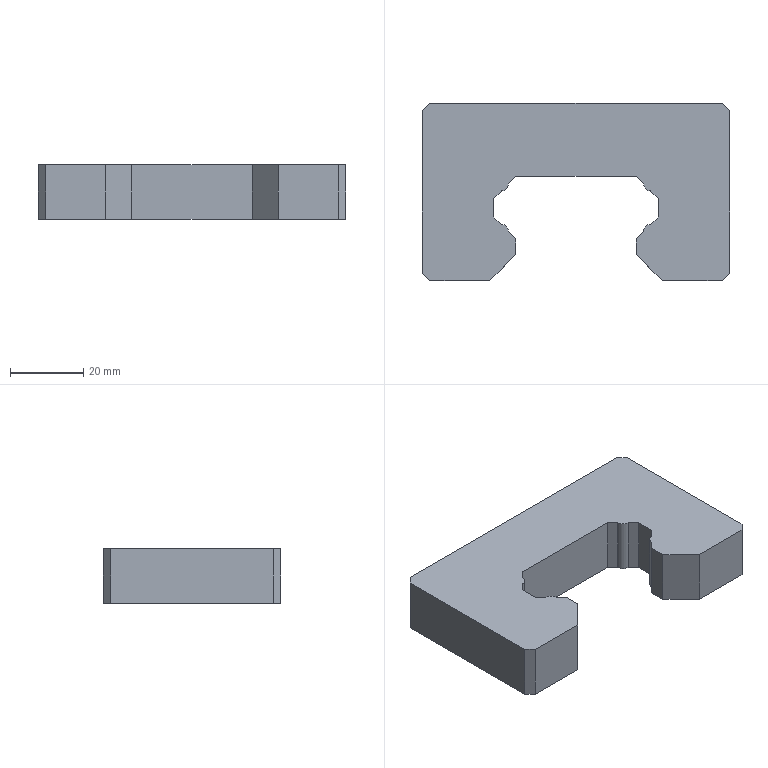Part | SolidWorks | features SplitBody 1 | 1 solid | 32 faces | box 84.105 x 48.48 x 15 mm | volume 44236 mm3 | plane 26 | cylinder 6 | commonest cylinder face diameters 3.924 x6
STEP:
#1=CARTESIAN_POINT('',(-18.51,13.429,79.55));
#2=VERTEX_POINT('',#1);
#3=CARTESIAN_POINT('',(-18.51,13.395,79.55));
#4=VERTEX_POINT('',#3);
#5=CARTESIAN_POINT('',(-20.471,13.429,79.55));
#6=DIRECTION('',(0.,0.,-1.));
#7=DIRECTION('',(-1.,0.,0.));
#8=AXIS2_PLACEMENT_3D('',#5,#6,#7);
#9=CIRCLE('',#8,1.962);
#10=EDGE_CURVE('',#2,#4,#9,.T.);
#11=ORIENTED_EDGE('',*,*,#10,.F.);
#12=CARTESIAN_POINT('',(-18.51,13.429,94.55));
#13=VERTEX_POINT('',#12);
#14=CARTESIAN_POINT('',(-18.51,13.429,79.55));
#15=DIRECTION('',(0.,0.,1.));
#16=VECTOR('',#15,1000.);
#17=LINE('',#14,#16);
#18=EDGE_CURVE('',#2,#13,#17,.T.);
#19=ORIENTED_EDGE('',*,*,#18,.T.);
#20=CARTESIAN_POINT('',(-18.51,13.395,94.55));
#21=VERTEX_POINT('',#20);
#22=CARTESIAN_POINT('',(-20.471,13.429,94.55));
#23=DIRECTION('',(0.,0.,-1.));
#24=DIRECTION('',(-1.,0.,0.));
#25=AXIS2_PLACEMENT_3D('',#22,#23,#24);
#26=CIRCLE('',#25,1.962);
#27=EDGE_CURVE('',#13,#21,#26,.T.);
#28=ORIENTED_EDGE('',*,*,#27,.T.);
#29=CARTESIAN_POINT('',(-18.51,13.395,79.55));
#30=DIRECTION('',(0.,0.,1.));
#31=VECTOR('',#30,1000.);
#32=LINE('',#29,#31);
#33=EDGE_CURVE('',#4,#21,#32,.T.);
#34=ORIENTED_EDGE('',*,*,#33,.F.);
#35=EDGE_LOOP('',(#11,#19,#28,#34));
#36=FACE_OUTER_BOUND('',#35,.T.);
#37=CARTESIAN_POINT('',(-20.471,13.429,79.55));
#38=DIRECTION('',(0.,0.,1.));
#39=DIRECTION('',(1.,0.,0.));
#40=AXIS2_PLACEMENT_3D('',#37,#38,#39);
#41=CYLINDRICAL_SURFACE('',#40,1.962);
#42=ADVANCED_FACE('',(#36),#41,.T.);
#43=CARTESIAN_POINT('',(-18.51,26.471,79.55));
#44=VERTEX_POINT('',#43);
#45=CARTESIAN_POINT('',(-20.505,24.51,79.55));
#46=VERTEX_POINT('',#45);
#47=CARTESIAN_POINT('',(-20.471,26.471,79.55));
#48=DIRECTION('',(0.,0.,-1.));
#49=DIRECTION('',(-1.,0.,0.));
#50=AXIS2_PLACEMENT_3D('',#47,#48,#49);
#51=CIRCLE('',#50,1.962);
#52=EDGE_CURVE('',#44,#46,#51,.T.);
#53=ORIENTED_EDGE('',*,*,#52,.F.);
#54=CARTESIAN_POINT('',(-18.51,26.471,94.55));
#55=VERTEX_POINT('',#54);
#56=CARTESIAN_POINT('',(-18.51,26.471,79.55));
#57=DIRECTION('',(0.,0.,1.));
#58=VECTOR('',#57,1000.);
#59=LINE('',#56,#58);
#60=EDGE_CURVE('',#44,#55,#59,.T.);
#61=ORIENTED_EDGE('',*,*,#60,.T.);
#62=CARTESIAN_POINT('',(-20.505,24.51,94.55));
#63=VERTEX_POINT('',#62);
#64=CARTESIAN_POINT('',(-20.471,26.471,94.55));
#65=DIRECTION('',(0.,0.,-1.));
#66=DIRECTION('',(-1.,0.,0.));
#67=AXIS2_PLACEMENT_3D('',#64,#65,#66);
#68=CIRCLE('',#67,1.962);
#69=EDGE_CURVE('',#55,#63,#68,.T.);
#70=ORIENTED_EDGE('',*,*,#69,.T.);
#71=CARTESIAN_POINT('',(-20.505,24.51,79.55));
#72=DIRECTION('',(0.,0.,1.));
#73=VECTOR('',#72,1000.);
#74=LINE('',#71,#73);
#75=EDGE_CURVE('',#46,#63,#74,.T.);
#76=ORIENTED_EDGE('',*,*,#75,.F.);
#77=EDGE_LOOP('',(#53,#61,#70,#76));
#78=FACE_OUTER_BOUND('',#77,.T.);
#79=CARTESIAN_POINT('',(-20.471,26.471,79.55));
#80=DIRECTION('',(0.,0.,1.));
#81=DIRECTION('',(1.,0.,0.));
#82=AXIS2_PLACEMENT_3D('',#79,#80,#81);
#83=CYLINDRICAL_SURFACE('',#82,1.962);
#84=ADVANCED_FACE('',(#78),#83,.T.);
#85=CARTESIAN_POINT('',(-16.515,11.4,94.55));
#86=VERTEX_POINT('',#85);
#87=CARTESIAN_POINT('',(-16.515,7.11,94.55));
#88=VERTEX_POINT('',#87);
#89=CARTESIAN_POINT('',(-16.515,11.4,94.55));
#90=DIRECTION('',(0.,-1.,0.));
#91=VECTOR('',#90,1000.);
#92=LINE('',#89,#91);
#93=EDGE_CURVE('',#86,#88,#92,.T.);
#94=ORIENTED_EDGE('',*,*,#93,.T.);
#95=CARTESIAN_POINT('',(-16.515,7.11,79.55));
#96=VERTEX_POINT('',#95);
#97=CARTESIAN_POINT('',(-16.515,7.11,79.55));
#98=DIRECTION('',(0.,0.,1.));
#99=VECTOR('',#98,1000.);
#100=LINE('',#97,#99);
#101=EDGE_CURVE('',#96,#88,#100,.T.);
#102=ORIENTED_EDGE('',*,*,#101,.F.);
#103=CARTESIAN_POINT('',(-16.515,11.4,79.55));
#104=VERTEX_POINT('',#103);
#105=CARTESIAN_POINT('',(-16.515,11.4,79.55));
#106=DIRECTION('',(0.,-1.,0.));
#107=VECTOR('',#106,1000.);
#108=LINE('',#105,#107);
#109=EDGE_CURVE('',#104,#96,#108,.T.);
#110=ORIENTED_EDGE('',*,*,#109,.F.);
#111=CARTESIAN_POINT('',(-16.515,11.4,79.55));
#112=DIRECTION('',(0.,0.,1.));
#113=VECTOR('',#112,1000.);
#114=LINE('',#111,#113);
#115=EDGE_CURVE('',#104,#86,#114,.T.);
#116=ORIENTED_EDGE('',*,*,#115,.T.);
#117=EDGE_LOOP('',(#94,#102,#110,#116));
#118=FACE_OUTER_BOUND('',#117,.T.);
#119=CARTESIAN_POINT('',(-16.515,11.4,79.55));
#120=DIRECTION('',(-1.,0.,0.));
#121=DIRECTION('',(0.,-1.,0.));
#122=AXIS2_PLACEMENT_3D('',#119,#120,#121);
#123=PLANE('',#122);
#124=ADVANCED_FACE('',(#118),#123,.F.);
#125=CARTESIAN_POINT('',(-23.625,0.,94.55));
#126=VERTEX_POINT('',#125);
#127=CARTESIAN_POINT('',(-16.515,7.11,94.55));
#128=DIRECTION('',(-0.7071,-0.7071,0.));
#129=VECTOR('',#128,1000.);
#130=LINE('',#127,#129);
#131=EDGE_CURVE('',#88,#126,#130,.T.);
#132=ORIENTED_EDGE('',*,*,#131,.T.);
#133=CARTESIAN_POINT('',(-23.625,0.,79.55));
#134=VERTEX_POINT('',#133);
#135=CARTESIAN_POINT('',(-23.625,0.,79.55));
#136=DIRECTION('',(0.,0.,1.));
#137=VECTOR('',#136,1000.);
#138=LINE('',#135,#137);
#139=EDGE_CURVE('',#134,#126,#138,.T.);
#140=ORIENTED_EDGE('',*,*,#139,.F.);
#141=CARTESIAN_POINT('',(-16.515,7.11,79.55));
#142=DIRECTION('',(-0.7071,-0.7071,0.));
#143=VECTOR('',#142,1000.);
#144=LINE('',#141,#143);
#145=EDGE_CURVE('',#96,#134,#144,.T.);
#146=ORIENTED_EDGE('',*,*,#145,.F.);
#147=ORIENTED_EDGE('',*,*,#101,.T.);
#148=EDGE_LOOP('',(#132,#140,#146,#147));
#149=FACE_OUTER_BOUND('',#148,.T.);
#150=CARTESIAN_POINT('',(-16.515,7.11,79.55));
#151=DIRECTION('',(-0.7071,0.7071,0.));
#152=DIRECTION('',(-0.7071,-0.7071,0.));
#153=AXIS2_PLACEMENT_3D('',#150,#151,#152);
#154=PLANE('',#153);
#155=ADVANCED_FACE('',(#149),#154,.F.);
#156=CARTESIAN_POINT('',(-40.05,0.,94.55));
#157=VERTEX_POINT('',#156);
#158=CARTESIAN_POINT('',(-23.625,0.,94.55));
#159=DIRECTION('',(-1.,0.,0.));
#160=VECTOR('',#159,1000.);
#161=LINE('',#158,#160);
#162=EDGE_CURVE('',#126,#157,#161,.T.);
#163=ORIENTED_EDGE('',*,*,#162,.T.);
#164=CARTESIAN_POINT('',(-40.05,0.,79.55));
#165=VERTEX_POINT('',#164);
#166=CARTESIAN_POINT('',(-40.05,0.,79.55));
#167=DIRECTION('',(0.,0.,1.));
#168=VECTOR('',#167,1000.);
#169=LINE('',#166,#168);
#170=EDGE_CURVE('',#165,#157,#169,.T.);
#171=ORIENTED_EDGE('',*,*,#170,.F.);
#172=CARTESIAN_POINT('',(-23.625,0.,79.55));
#173=DIRECTION('',(-1.,0.,0.));
#174=VECTOR('',#173,1000.);
#175=LINE('',#172,#174);
#176=EDGE_CURVE('',#134,#165,#175,.T.);
#177=ORIENTED_EDGE('',*,*,#176,.F.);
#178=ORIENTED_EDGE('',*,*,#139,.T.);
#179=EDGE_LOOP('',(#163,#171,#177,#178));
#180=FACE_OUTER_BOUND('',#179,.T.);
#181=CARTESIAN_POINT('',(-23.625,0.,79.55));
#182=DIRECTION('',(0.,1.,0.));
#183=DIRECTION('',(-1.,0.,0.));
#184=AXIS2_PLACEMENT_3D('',#181,#182,#183);
#185=PLANE('',#184);
#186=ADVANCED_FACE('',(#180),#185,.F.);
#187=CARTESIAN_POINT('',(-42.053,2.002,94.55));
#188=VERTEX_POINT('',#187);
#189=CARTESIAN_POINT('',(-40.05,0.,94.55));
#190=DIRECTION('',(-0.7071,0.7071,0.));
#191=VECTOR('',#190,1000.);
#192=LINE('',#189,#191);
#193=EDGE_CURVE('',#157,#188,#192,.T.);
#194=ORIENTED_EDGE('',*,*,#193,.T.);
#195=CARTESIAN_POINT('',(-42.053,2.002,79.55));
#196=VERTEX_POINT('',#195);
#197=CARTESIAN_POINT('',(-42.053,2.002,79.55));
#198=DIRECTION('',(0.,0.,1.));
#199=VECTOR('',#198,1000.);
#200=LINE('',#197,#199);
#201=EDGE_CURVE('',#196,#188,#200,.T.);
#202=ORIENTED_EDGE('',*,*,#201,.F.);
#203=CARTESIAN_POINT('',(-40.05,0.,79.55));
#204=DIRECTION('',(-0.7071,0.7071,0.));
#205=VECTOR('',#204,1000.);
#206=LINE('',#203,#205);
#207=EDGE_CURVE('',#165,#196,#206,.T.);
#208=ORIENTED_EDGE('',*,*,#207,.F.);
#209=ORIENTED_EDGE('',*,*,#170,.T.);
#210=EDGE_LOOP('',(#194,#202,#208,#209));
#211=FACE_OUTER_BOUND('',#210,.T.);
#212=CARTESIAN_POINT('',(-40.05,0.,79.55));
#213=DIRECTION('',(0.7071,0.7071,0.));
#214=DIRECTION('',(-0.7071,0.7071,0.));
#215=AXIS2_PLACEMENT_3D('',#212,#213,#214);
#216=PLANE('',#215);
#217=ADVANCED_FACE('',(#211),#216,.F.);
#218=CARTESIAN_POINT('',(-42.053,46.477,94.55));
#219=VERTEX_POINT('',#218);
#220=CARTESIAN_POINT('',(-42.053,2.002,94.55));
#221=DIRECTION('',(0.,1.,0.));
#222=VECTOR('',#221,1000.);
#223=LINE('',#220,#222);
#224=EDGE_CURVE('',#188,#219,#223,.T.);
#225=ORIENTED_EDGE('',*,*,#224,.T.);
#226=CARTESIAN_POINT('',(-42.053,46.477,79.55));
#227=VERTEX_POINT('',#226);
#228=CARTESIAN_POINT('',(-42.053,46.477,79.55));
#229=DIRECTION('',(0.,0.,1.));
#230=VECTOR('',#229,1000.);
#231=LINE('',#228,#230);
#232=EDGE_CURVE('',#227,#219,#231,.T.);
#233=ORIENTED_EDGE('',*,*,#232,.F.);
#234=CARTESIAN_POINT('',(-42.053,2.002,79.55));
#235=DIRECTION('',(0.,1.,0.));
#236=VECTOR('',#235,1000.);
#237=LINE('',#234,#236);
#238=EDGE_CURVE('',#196,#227,#237,.T.);
#239=ORIENTED_EDGE('',*,*,#238,.F.);
#240=ORIENTED_EDGE('',*,*,#201,.T.);
#241=EDGE_LOOP('',(#225,#233,#239,#240));
#242=FACE_OUTER_BOUND('',#241,.T.);
#243=CARTESIAN_POINT('',(-42.053,2.002,79.55));
#244=DIRECTION('',(1.,0.,0.));
#245=DIRECTION('',(0.,0.,-1.));
#246=AXIS2_PLACEMENT_3D('',#243,#244,#245);
#247=PLANE('',#246);
#248=ADVANCED_FACE('',(#242),#247,.F.);
#249=CARTESIAN_POINT('',(-40.05,48.48,94.55));
#250=VERTEX_POINT('',#249);
#251=CARTESIAN_POINT('',(-42.053,46.477,94.55));
#252=DIRECTION('',(0.7071,0.7071,0.));
#253=VECTOR('',#252,1000.);
#254=LINE('',#251,#253);
#255=EDGE_CURVE('',#219,#250,#254,.T.);
#256=ORIENTED_EDGE('',*,*,#255,.T.);
#257=CARTESIAN_POINT('',(-40.05,48.48,79.55));
#258=VERTEX_POINT('',#257);
#259=CARTESIAN_POINT('',(-40.05,48.48,79.55));
#260=DIRECTION('',(0.,0.,1.));
#261=VECTOR('',#260,1000.);
#262=LINE('',#259,#261);
#263=EDGE_CURVE('',#258,#250,#262,.T.);
#264=ORIENTED_EDGE('',*,*,#263,.F.);
#265=CARTESIAN_POINT('',(-42.053,46.477,79.55));
#266=DIRECTION('',(0.7071,0.7071,0.));
#267=VECTOR('',#266,1000.);
#268=LINE('',#265,#267);
#269=EDGE_CURVE('',#227,#258,#268,.T.);
#270=ORIENTED_EDGE('',*,*,#269,.F.);
#271=ORIENTED_EDGE('',*,*,#232,.T.);
#272=EDGE_LOOP('',(#256,#264,#270,#271));
#273=FACE_OUTER_BOUND('',#272,.T.);
#274=CARTESIAN_POINT('',(-42.053,46.477,79.55));
#275=DIRECTION('',(0.7071,-0.7071,0.));
#276=DIRECTION('',(0.7071,0.7071,0.));
#277=AXIS2_PLACEMENT_3D('',#274,#275,#276);
#278=PLANE('',#277);
#279=ADVANCED_FACE('',(#273),#278,.F.);
#280=CARTESIAN_POINT('',(40.05,48.48,94.55));
#281=VERTEX_POINT('',#280);
#282=CARTESIAN_POINT('',(-40.05,48.48,94.55));
#283=DIRECTION('',(1.,0.,0.));
#284=VECTOR('',#283,1000.);
#285=LINE('',#282,#284);
#286=EDGE_CURVE('',#250,#281,#285,.T.);
#287=ORIENTED_EDGE('',*,*,#286,.T.);
#288=CARTESIAN_POINT('',(40.05,48.48,79.55));
#289=VERTEX_POINT('',#288);
#290=CARTESIAN_POINT('',(40.05,48.48,79.55));
#291=DIRECTION('',(0.,0.,1.));
#292=VECTOR('',#291,1000.);
#293=LINE('',#290,#292);
#294=EDGE_CURVE('',#289,#281,#293,.T.);
#295=ORIENTED_EDGE('',*,*,#294,.F.);
#296=CARTESIAN_POINT('',(-40.05,48.48,79.55));
#297=DIRECTION('',(1.,0.,0.));
#298=VECTOR('',#297,1000.);
#299=LINE('',#296,#298);
#300=EDGE_CURVE('',#258,#289,#299,.T.);
#301=ORIENTED_EDGE('',*,*,#300,.F.);
#302=ORIENTED_EDGE('',*,*,#263,.T.);
#303=EDGE_LOOP('',(#287,#295,#301,#302));
#304=FACE_OUTER_BOUND('',#303,.T.);
#305=CARTESIAN_POINT('',(-40.05,48.48,79.55));
#306=DIRECTION('',(0.,-1.,0.));
#307=DIRECTION('',(0.,0.,-1.));
#308=AXIS2_PLACEMENT_3D('',#305,#306,#307);
#309=PLANE('',#308);
#310=ADVANCED_FACE('',(#304),#309,.F.);
#311=CARTESIAN_POINT('',(42.053,46.477,94.55));
#312=VERTEX_POINT('',#311);
#313=CARTESIAN_POINT('',(40.05,48.48,94.55));
#314=DIRECTION('',(0.7071,-0.7071,0.));
#315=VECTOR('',#314,1000.);
#316=LINE('',#313,#315);
#317=EDGE_CURVE('',#281,#312,#316,.T.);
#318=ORIENTED_EDGE('',*,*,#317,.T.);
#319=CARTESIAN_POINT('',(42.053,46.477,79.55));
#320=VERTEX_POINT('',#319);
#321=CARTESIAN_POINT('',(42.053,46.477,79.55));
#322=DIRECTION('',(0.,0.,1.));
#323=VECTOR('',#322,1000.);
#324=LINE('',#321,#323);
#325=EDGE_CURVE('',#320,#312,#324,.T.);
#326=ORIENTED_EDGE('',*,*,#325,.F.);
#327=CARTESIAN_POINT('',(40.05,48.48,79.55));
#328=DIRECTION('',(0.7071,-0.7071,0.));
#329=VECTOR('',#328,1000.);
#330=LINE('',#327,#329);
#331=EDGE_CURVE('',#289,#320,#330,.T.);
#332=ORIENTED_EDGE('',*,*,#331,.F.);
#333=ORIENTED_EDGE('',*,*,#294,.T.);
#334=EDGE_LOOP('',(#318,#326,#332,#333));
#335=FACE_OUTER_BOUND('',#334,.T.);
#336=CARTESIAN_POINT('',(40.05,48.48,79.55));
#337=DIRECTION('',(-0.7071,-0.7071,0.));
#338=DIRECTION('',(0.7071,-0.7071,0.));
#339=AXIS2_PLACEMENT_3D('',#336,#337,#338);
#340=PLANE('',#339);
#341=ADVANCED_FACE('',(#335),#340,.F.);
#342=CARTESIAN_POINT('',(42.053,2.002,94.55));
#343=VERTEX_POINT('',#342);
#344=CARTESIAN_POINT('',(42.053,46.477,94.55));
#345=DIRECTION('',(0.,-1.,0.));
#346=VECTOR('',#345,1000.);
#347=LINE('',#344,#346);
#348=EDGE_CURVE('',#312,#343,#347,.T.);
#349=ORIENTED_EDGE('',*,*,#348,.T.);
#350=CARTESIAN_POINT('',(42.053,2.002,79.55));
#351=VERTEX_POINT('',#350);
#352=CARTESIAN_POINT('',(42.053,2.002,79.55));
#353=DIRECTION('',(0.,0.,1.));
#354=VECTOR('',#353,1000.);
#355=LINE('',#352,#354);
#356=EDGE_CURVE('',#351,#343,#355,.T.);
#357=ORIENTED_EDGE('',*,*,#356,.F.);
#358=CARTESIAN_POINT('',(42.053,46.477,79.55));
#359=DIRECTION('',(0.,-1.,0.));
#360=VECTOR('',#359,1000.);
#361=LINE('',#358,#360);
#362=EDGE_CURVE('',#320,#351,#361,.T.);
#363=ORIENTED_EDGE('',*,*,#362,.F.);
#364=ORIENTED_EDGE('',*,*,#325,.T.);
#365=EDGE_LOOP('',(#349,#357,#363,#364));
#366=FACE_OUTER_BOUND('',#365,.T.);
#367=CARTESIAN_POINT('',(42.053,46.477,79.55));
#368=DIRECTION('',(-1.,0.,0.));
#369=DIRECTION('',(0.,0.,1.));
#370=AXIS2_PLACEMENT_3D('',#367,#368,#369);
#371=PLANE('',#370);
#372=ADVANCED_FACE('',(#366),#371,.F.);
#373=CARTESIAN_POINT('',(40.05,0.,94.55));
#374=VERTEX_POINT('',#373);
#375=CARTESIAN_POINT('',(42.053,2.002,94.55));
#376=DIRECTION('',(-0.7071,-0.7071,0.));
#377=VECTOR('',#376,1000.);
#378=LINE('',#375,#377);
#379=EDGE_CURVE('',#343,#374,#378,.T.);
#380=ORIENTED_EDGE('',*,*,#379,.T.);
#381=CARTESIAN_POINT('',(40.05,0.,79.55));
#382=VERTEX_POINT('',#381);
#383=CARTESIAN_POINT('',(40.05,0.,79.55));
#384=DIRECTION('',(0.,0.,1.));
#385=VECTOR('',#384,1000.);
#386=LINE('',#383,#385);
#387=EDGE_CURVE('',#382,#374,#386,.T.);
#388=ORIENTED_EDGE('',*,*,#387,.F.);
#389=CARTESIAN_POINT('',(42.053,2.002,79.55));
#390=DIRECTION('',(-0.7071,-0.7071,0.));
#391=VECTOR('',#390,1000.);
#392=LINE('',#389,#391);
#393=EDGE_CURVE('',#351,#382,#392,.T.);
#394=ORIENTED_EDGE('',*,*,#393,.F.);
#395=ORIENTED_EDGE('',*,*,#356,.T.);
#396=EDGE_LOOP('',(#380,#388,#394,#395));
#397=FACE_OUTER_BOUND('',#396,.T.);
#398=CARTESIAN_POINT('',(42.053,2.002,79.55));
#399=DIRECTION('',(-0.7071,0.7071,0.));
#400=DIRECTION('',(-0.7071,-0.7071,0.));
#401=AXIS2_PLACEMENT_3D('',#398,#399,#400);
#402=PLANE('',#401);
#403=ADVANCED_FACE('',(#397),#402,.F.);
#404=CARTESIAN_POINT('',(23.625,0.,94.55));
#405=VERTEX_POINT('',#404);
#406=CARTESIAN_POINT('',(40.05,0.,94.55));
#407=DIRECTION('',(-1.,0.,0.));
#408=VECTOR('',#407,1000.);
#409=LINE('',#406,#408);
#410=EDGE_CURVE('',#374,#405,#409,.T.);
#411=ORIENTED_EDGE('',*,*,#410,.T.);
#412=CARTESIAN_POINT('',(23.625,0.,79.55));
#413=VERTEX_POINT('',#412);
#414=CARTESIAN_POINT('',(23.625,0.,79.55));
#415=DIRECTION('',(0.,0.,1.));
#416=VECTOR('',#415,1000.);
#417=LINE('',#414,#416);
#418=EDGE_CURVE('',#413,#405,#417,.T.);
#419=ORIENTED_EDGE('',*,*,#418,.F.);
#420=CARTESIAN_POINT('',(40.05,0.,79.55));
#421=DIRECTION('',(-1.,0.,0.));
#422=VECTOR('',#421,1000.);
#423=LINE('',#420,#422);
#424=EDGE_CURVE('',#382,#413,#423,.T.);
#425=ORIENTED_EDGE('',*,*,#424,.F.);
#426=ORIENTED_EDGE('',*,*,#387,.T.);
#427=EDGE_LOOP('',(#411,#419,#425,#426));
#428=FACE_OUTER_BOUND('',#427,.T.);
#429=CARTESIAN_POINT('',(40.05,0.,79.55));
#430=DIRECTION('',(0.,1.,0.));
#431=DIRECTION('',(-1.,0.,0.));
#432=AXIS2_PLACEMENT_3D('',#429,#430,#431);
#433=PLANE('',#432);
#434=ADVANCED_FACE('',(#428),#433,.F.);
#435=CARTESIAN_POINT('',(16.515,7.11,94.55));
#436=VERTEX_POINT('',#435);
#437=CARTESIAN_POINT('',(23.625,0.,94.55));
#438=DIRECTION('',(-0.7071,0.7071,0.));
#439=VECTOR('',#438,1000.);
#440=LINE('',#437,#439);
#441=EDGE_CURVE('',#405,#436,#440,.T.);
#442=ORIENTED_EDGE('',*,*,#441,.T.);
#443=CARTESIAN_POINT('',(16.515,7.11,79.55));
#444=VERTEX_POINT('',#443);
#445=CARTESIAN_POINT('',(16.515,7.11,79.55));
#446=DIRECTION('',(0.,0.,1.));
#447=VECTOR('',#446,1000.);
#448=LINE('',#445,#447);
#449=EDGE_CURVE('',#444,#436,#448,.T.);
#450=ORIENTED_EDGE('',*,*,#449,.F.);
#451=CARTESIAN_POINT('',(23.625,0.,79.55));
#452=DIRECTION('',(-0.7071,0.7071,0.));
#453=VECTOR('',#452,1000.);
#454=LINE('',#451,#453);
#455=EDGE_CURVE('',#413,#444,#454,.T.);
#456=ORIENTED_EDGE('',*,*,#455,.F.);
#457=ORIENTED_EDGE('',*,*,#418,.T.);
#458=EDGE_LOOP('',(#442,#450,#456,#457));
#459=FACE_OUTER_BOUND('',#458,.T.);
#460=CARTESIAN_POINT('',(23.625,0.,79.55));
#461=DIRECTION('',(0.7071,0.7071,0.));
#462=DIRECTION('',(-0.7071,0.7071,0.));
#463=AXIS2_PLACEMENT_3D('',#460,#461,#462);
#464=PLANE('',#463);
#465=ADVANCED_FACE('',(#459),#464,.F.);
#466=CARTESIAN_POINT('',(16.515,11.4,94.55));
#467=VERTEX_POINT('',#466);
#468=CARTESIAN_POINT('',(16.515,7.11,94.55));
#469=DIRECTION('',(0.,1.,0.));
#470=VECTOR('',#469,1000.);
#471=LINE('',#468,#470);
#472=EDGE_CURVE('',#436,#467,#471,.T.);
#473=ORIENTED_EDGE('',*,*,#472,.T.);
#474=CARTESIAN_POINT('',(16.515,11.4,79.55));
#475=VERTEX_POINT('',#474);
#476=CARTESIAN_POINT('',(16.515,11.4,79.55));
#477=DIRECTION('',(0.,0.,1.));
#478=VECTOR('',#477,1000.);
#479=LINE('',#476,#478);
#480=EDGE_CURVE('',#475,#467,#479,.T.);
#481=ORIENTED_EDGE('',*,*,#480,.F.);
#482=CARTESIAN_POINT('',(16.515,7.11,79.55));
#483=DIRECTION('',(0.,1.,0.));
#484=VECTOR('',#483,1000.);
#485=LINE('',#482,#484);
#486=EDGE_CURVE('',#444,#475,#485,.T.);
#487=ORIENTED_EDGE('',*,*,#486,.F.);
#488=ORIENTED_EDGE('',*,*,#449,.T.);
#489=EDGE_LOOP('',(#473,#481,#487,#488));
#490=FACE_OUTER_BOUND('',#489,.T.);
#491=CARTESIAN_POINT('',(16.515,7.11,79.55));
#492=DIRECTION('',(1.,0.,0.));
#493=DIRECTION('',(0.,1.,0.));
#494=AXIS2_PLACEMENT_3D('',#491,#492,#493);
#495=PLANE('',#494);
#496=ADVANCED_FACE('',(#490),#495,.F.);
#497=CARTESIAN_POINT('',(18.51,13.395,94.55));
#498=VERTEX_POINT('',#497);
#499=CARTESIAN_POINT('',(16.515,11.4,94.55));
#500=DIRECTION('',(0.7071,0.7071,0.));
#501=VECTOR('',#500,1000.);
#502=LINE('',#499,#501);
#503=EDGE_CURVE('',#467,#498,#502,.T.);
#504=ORIENTED_EDGE('',*,*,#503,.T.);
#505=CARTESIAN_POINT('',(18.51,13.395,79.55));
#506=VERTEX_POINT('',#505);
#507=CARTESIAN_POINT('',(18.51,13.395,79.55));
#508=DIRECTION('',(0.,0.,1.));
#509=VECTOR('',#508,1000.);
#510=LINE('',#507,#509);
#511=EDGE_CURVE('',#506,#498,#510,.T.);
#512=ORIENTED_EDGE('',*,*,#511,.F.);
#513=CARTESIAN_POINT('',(16.515,11.4,79.55));
#514=DIRECTION('',(0.7071,0.7071,0.));
#515=VECTOR('',#514,1000.);
#516=LINE('',#513,#515);
#517=EDGE_CURVE('',#475,#506,#516,.T.);
#518=ORIENTED_EDGE('',*,*,#517,.F.);
#519=ORIENTED_EDGE('',*,*,#480,.T.);
#520=EDGE_LOOP('',(#504,#512,#518,#519));
#521=FACE_OUTER_BOUND('',#520,.T.);
#522=CARTESIAN_POINT('',(16.515,11.4,79.55));
#523=DIRECTION('',(0.7071,-0.7071,0.));
#524=DIRECTION('',(0.7071,0.7071,0.));
#525=AXIS2_PLACEMENT_3D('',#522,#523,#524);
#526=PLANE('',#525);
#527=ADVANCED_FACE('',(#521),#526,.F.);
#528=CARTESIAN_POINT('',(20.505,15.39,94.55));
#529=VERTEX_POINT('',#528);
#530=CARTESIAN_POINT('',(20.471,13.429,94.55));
#531=DIRECTION('',(0.,0.,-1.));
#532=DIRECTION('',(-1.,0.,0.));
#533=AXIS2_PLACEMENT_3D('',#530,#531,#532);
#534=CIRCLE('',#533,1.962);
#535=EDGE_CURVE('',#498,#529,#534,.T.);
#536=ORIENTED_EDGE('',*,*,#535,.T.);
#537=CARTESIAN_POINT('',(20.505,15.39,79.55));
#538=VERTEX_POINT('',#537);
#539=CARTESIAN_POINT('',(20.505,15.39,79.55));
#540=DIRECTION('',(0.,0.,1.));
#541=VECTOR('',#540,1000.);
#542=LINE('',#539,#541);
#543=EDGE_CURVE('',#538,#529,#542,.T.);
#544=ORIENTED_EDGE('',*,*,#543,.F.);
#545=CARTESIAN_POINT('',(20.471,13.429,79.55));
#546=DIRECTION('',(0.,0.,-1.));
#547=DIRECTION('',(-1.,0.,0.));
#548=AXIS2_PLACEMENT_3D('',#545,#546,#547);
#549=CIRCLE('',#548,1.962);
#550=EDGE_CURVE('',#506,#538,#549,.T.);
#551=ORIENTED_EDGE('',*,*,#550,.F.);
#552=ORIENTED_EDGE('',*,*,#511,.T.);
#553=EDGE_LOOP('',(#536,#544,#551,#552));
#554=FACE_OUTER_BOUND('',#553,.T.);
#555=CARTESIAN_POINT('',(20.471,13.429,79.55));
#556=DIRECTION('',(0.,0.,1.));
#557=DIRECTION('',(1.,0.,0.));
#558=AXIS2_PLACEMENT_3D('',#555,#556,#557);
#559=CYLINDRICAL_SURFACE('',#558,1.962);
#560=ADVANCED_FACE('',(#554),#559,.T.);
#561=CARTESIAN_POINT('',(22.5,17.385,94.55));
#562=VERTEX_POINT('',#561);
#563=CARTESIAN_POINT('',(20.505,15.39,94.55));
#564=DIRECTION('',(0.7071,0.7071,0.));
#565=VECTOR('',#564,1000.);
#566=LINE('',#563,#565);
#567=EDGE_CURVE('',#529,#562,#566,.T.);
#568=ORIENTED_EDGE('',*,*,#567,.T.);
#569=CARTESIAN_POINT('',(22.5,17.385,79.55));
#570=VERTEX_POINT('',#569);
#571=CARTESIAN_POINT('',(22.5,17.385,79.55));
#572=DIRECTION('',(0.,0.,1.));
#573=VECTOR('',#572,1000.);
#574=LINE('',#571,#573);
#575=EDGE_CURVE('',#570,#562,#574,.T.);
#576=ORIENTED_EDGE('',*,*,#575,.F.);
#577=CARTESIAN_POINT('',(20.505,15.39,79.55));
#578=DIRECTION('',(0.7071,0.7071,0.));
#579=VECTOR('',#578,1000.);
#580=LINE('',#577,#579);
#581=EDGE_CURVE('',#538,#570,#580,.T.);
#582=ORIENTED_EDGE('',*,*,#581,.F.);
#583=ORIENTED_EDGE('',*,*,#543,.T.);
#584=EDGE_LOOP('',(#568,#576,#582,#583));
#585=FACE_OUTER_BOUND('',#584,.T.);
#586=CARTESIAN_POINT('',(20.505,15.39,79.55));
#587=DIRECTION('',(0.7071,-0.7071,0.));
#588=DIRECTION('',(0.7071,0.7071,0.));
#589=AXIS2_PLACEMENT_3D('',#586,#587,#588);
#590=PLANE('',#589);
#591=ADVANCED_FACE('',(#585),#590,.F.);
#592=CARTESIAN_POINT('',(22.5,22.515,94.55));
#593=VERTEX_POINT('',#592);
#594=CARTESIAN_POINT('',(22.5,17.385,94.55));
#595=DIRECTION('',(0.,1.,0.));
#596=VECTOR('',#595,1000.);
#597=LINE('',#594,#596);
#598=EDGE_CURVE('',#562,#593,#597,.T.);
#599=ORIENTED_EDGE('',*,*,#598,.T.);
#600=CARTESIAN_POINT('',(22.5,22.515,79.55));
#601=VERTEX_POINT('',#600);
#602=CARTESIAN_POINT('',(22.5,22.515,79.55));
#603=DIRECTION('',(0.,0.,1.));
#604=VECTOR('',#603,1000.);
#605=LINE('',#602,#604);
#606=EDGE_CURVE('',#601,#593,#605,.T.);
#607=ORIENTED_EDGE('',*,*,#606,.F.);
#608=CARTESIAN_POINT('',(22.5,17.385,79.55));
#609=DIRECTION('',(0.,1.,0.));
#610=VECTOR('',#609,1000.);
#611=LINE('',#608,#610);
#612=EDGE_CURVE('',#570,#601,#611,.T.);
#613=ORIENTED_EDGE('',*,*,#612,.F.);
#614=ORIENTED_EDGE('',*,*,#575,.T.);
#615=EDGE_LOOP('',(#599,#607,#613,#614));
#616=FACE_OUTER_BOUND('',#615,.T.);
#617=CARTESIAN_POINT('',(22.5,17.385,79.55));
#618=DIRECTION('',(1.,0.,0.));
#619=DIRECTION('',(0.,0.,-1.));
#620=AXIS2_PLACEMENT_3D('',#617,#618,#619);
#621=PLANE('',#620);
#622=ADVANCED_FACE('',(#616),#621,.F.);
#623=CARTESIAN_POINT('',(20.505,24.51,94.55));
#624=VERTEX_POINT('',#623);
#625=CARTESIAN_POINT('',(22.5,22.515,94.55));
#626=DIRECTION('',(-0.7071,0.7071,0.));
#627=VECTOR('',#626,1000.);
#628=LINE('',#625,#627);
#629=EDGE_CURVE('',#593,#624,#628,.T.);
#630=ORIENTED_EDGE('',*,*,#629,.T.);
#631=CARTESIAN_POINT('',(20.505,24.51,79.55));
#632=VERTEX_POINT('',#631);
#633=CARTESIAN_POINT('',(20.505,24.51,79.55));
#634=DIRECTION('',(0.,0.,1.));
#635=VECTOR('',#634,1000.);
#636=LINE('',#633,#635);
#637=EDGE_CURVE('',#632,#624,#636,.T.);
#638=ORIENTED_EDGE('',*,*,#637,.F.);
#639=CARTESIAN_POINT('',(22.5,22.515,79.55));
#640=DIRECTION('',(-0.7071,0.7071,0.));
#641=VECTOR('',#640,1000.);
#642=LINE('',#639,#641);
#643=EDGE_CURVE('',#601,#632,#642,.T.);
#644=ORIENTED_EDGE('',*,*,#643,.F.);
#645=ORIENTED_EDGE('',*,*,#606,.T.);
#646=EDGE_LOOP('',(#630,#638,#644,#645));
#647=FACE_OUTER_BOUND('',#646,.T.);
#648=CARTESIAN_POINT('',(22.5,22.515,79.55));
#649=DIRECTION('',(0.7071,0.7071,0.));
#650=DIRECTION('',(-0.7071,0.7071,0.));
#651=AXIS2_PLACEMENT_3D('',#648,#649,#650);
#652=PLANE('',#651);
#653=ADVANCED_FACE('',(#647),#652,.F.);
#654=CARTESIAN_POINT('',(18.51,26.505,94.55));
#655=VERTEX_POINT('',#654);
#656=CARTESIAN_POINT('',(20.471,26.471,94.55));
#657=DIRECTION('',(0.,0.,-1.));
#658=DIRECTION('',(-1.,0.,0.));
#659=AXIS2_PLACEMENT_3D('',#656,#657,#658);
#660=CIRCLE('',#659,1.962);
#661=EDGE_CURVE('',#624,#655,#660,.T.);
#662=ORIENTED_EDGE('',*,*,#661,.T.);
#663=CARTESIAN_POINT('',(18.51,26.505,79.55));
#664=VERTEX_POINT('',#663);
#665=CARTESIAN_POINT('',(18.51,26.505,79.55));
#666=DIRECTION('',(0.,0.,1.));
#667=VECTOR('',#666,1000.);
#668=LINE('',#665,#667);
#669=EDGE_CURVE('',#664,#655,#668,.T.);
#670=ORIENTED_EDGE('',*,*,#669,.F.);
#671=CARTESIAN_POINT('',(20.471,26.471,79.55));
#672=DIRECTION('',(0.,0.,-1.));
#673=DIRECTION('',(-1.,0.,0.));
#674=AXIS2_PLACEMENT_3D('',#671,#672,#673);
#675=CIRCLE('',#674,1.962);
#676=EDGE_CURVE('',#632,#664,#675,.T.);
#677=ORIENTED_EDGE('',*,*,#676,.F.);
#678=ORIENTED_EDGE('',*,*,#637,.T.);
#679=EDGE_LOOP('',(#662,#670,#677,#678));
#680=FACE_OUTER_BOUND('',#679,.T.);
#681=CARTESIAN_POINT('',(20.471,26.471,79.55));
#682=DIRECTION('',(0.,0.,1.));
#683=DIRECTION('',(1.,0.,0.));
#684=AXIS2_PLACEMENT_3D('',#681,#682,#683);
#685=CYLINDRICAL_SURFACE('',#684,1.962);
#686=ADVANCED_FACE('',(#680),#685,.T.);
#687=CARTESIAN_POINT('',(16.515,28.5,94.55));
#688=VERTEX_POINT('',#687);
#689=CARTESIAN_POINT('',(18.51,26.505,94.55));
#690=DIRECTION('',(-0.7071,0.7071,0.));
#691=VECTOR('',#690,1000.);
#692=LINE('',#689,#691);
#693=EDGE_CURVE('',#655,#688,#692,.T.);
#694=ORIENTED_EDGE('',*,*,#693,.T.);
#695=CARTESIAN_POINT('',(16.515,28.5,79.55));
#696=VERTEX_POINT('',#695);
#697=CARTESIAN_POINT('',(16.515,28.5,79.55));
#698=DIRECTION('',(0.,0.,1.));
#699=VECTOR('',#698,1000.);
#700=LINE('',#697,#699);
#701=EDGE_CURVE('',#696,#688,#700,.T.);
#702=ORIENTED_EDGE('',*,*,#701,.F.);
#703=CARTESIAN_POINT('',(18.51,26.505,79.55));
#704=DIRECTION('',(-0.7071,0.7071,0.));
#705=VECTOR('',#704,1000.);
#706=LINE('',#703,#705);
#707=EDGE_CURVE('',#664,#696,#706,.T.);
#708=ORIENTED_EDGE('',*,*,#707,.F.);
#709=ORIENTED_EDGE('',*,*,#669,.T.);
#710=EDGE_LOOP('',(#694,#702,#708,#709));
#711=FACE_OUTER_BOUND('',#710,.T.);
#712=CARTESIAN_POINT('',(18.51,26.505,79.55));
#713=DIRECTION('',(0.7071,0.7071,0.));
#714=DIRECTION('',(-0.7071,0.7071,0.));
#715=AXIS2_PLACEMENT_3D('',#712,#713,#714);
#716=PLANE('',#715);
#717=ADVANCED_FACE('',(#711),#716,.F.);
#718=CARTESIAN_POINT('',(-16.515,28.5,94.55));
#719=VERTEX_POINT('',#718);
#720=CARTESIAN_POINT('',(16.515,28.5,94.55));
#721=DIRECTION('',(-1.,0.,0.));
#722=VECTOR('',#721,1000.);
#723=LINE('',#720,#722);
#724=EDGE_CURVE('',#688,#719,#723,.T.);
#725=ORIENTED_EDGE('',*,*,#724,.T.);
#726=CARTESIAN_POINT('',(-16.515,28.5,79.55));
#727=VERTEX_POINT('',#726);
#728=CARTESIAN_POINT('',(-16.515,28.5,79.55));
#729=DIRECTION('',(0.,0.,1.));
#730=VECTOR('',#729,1000.);
#731=LINE('',#728,#730);
#732=EDGE_CURVE('',#727,#719,#731,.T.);
#733=ORIENTED_EDGE('',*,*,#732,.F.);
#734=CARTESIAN_POINT('',(16.515,28.5,79.55));
#735=DIRECTION('',(-1.,0.,0.));
#736=VECTOR('',#735,1000.);
#737=LINE('',#734,#736);
#738=EDGE_CURVE('',#696,#727,#737,.T.);
#739=ORIENTED_EDGE('',*,*,#738,.F.);
#740=ORIENTED_EDGE('',*,*,#701,.T.);
#741=EDGE_LOOP('',(#725,#733,#739,#740));
#742=FACE_OUTER_BOUND('',#741,.T.);
#743=CARTESIAN_POINT('',(16.515,28.5,79.55));
#744=DIRECTION('',(0.,1.,0.));
#745=DIRECTION('',(0.,0.,1.));
#746=AXIS2_PLACEMENT_3D('',#743,#744,#745);
#747=PLANE('',#746);
#748=ADVANCED_FACE('',(#742),#747,.F.);
#749=CARTESIAN_POINT('',(-18.51,26.505,94.55));
#750=VERTEX_POINT('',#749);
#751=CARTESIAN_POINT('',(-16.515,28.5,94.55));
#752=DIRECTION('',(-0.7071,-0.7071,0.));
#753=VECTOR('',#752,1000.);
#754=LINE('',#751,#753);
#755=EDGE_CURVE('',#719,#750,#754,.T.);
#756=ORIENTED_EDGE('',*,*,#755,.T.);
#757=CARTESIAN_POINT('',(-18.51,26.505,79.55));
#758=VERTEX_POINT('',#757);
#759=CARTESIAN_POINT('',(-18.51,26.505,79.55));
#760=DIRECTION('',(0.,0.,1.));
#761=VECTOR('',#760,1000.);
#762=LINE('',#759,#761);
#763=EDGE_CURVE('',#758,#750,#762,.T.);
#764=ORIENTED_EDGE('',*,*,#763,.F.);
#765=CARTESIAN_POINT('',(-16.515,28.5,79.55));
#766=DIRECTION('',(-0.7071,-0.7071,0.));
#767=VECTOR('',#766,1000.);
#768=LINE('',#765,#767);
#769=EDGE_CURVE('',#727,#758,#768,.T.);
#770=ORIENTED_EDGE('',*,*,#769,.F.);
#771=ORIENTED_EDGE('',*,*,#732,.T.);
#772=EDGE_LOOP('',(#756,#764,#770,#771));
#773=FACE_OUTER_BOUND('',#772,.T.);
#774=CARTESIAN_POINT('',(-16.515,28.5,79.55));
#775=DIRECTION('',(-0.7071,0.7071,0.));
#776=DIRECTION('',(-0.7071,-0.7071,0.));
#777=AXIS2_PLACEMENT_3D('',#774,#775,#776);
#778=PLANE('',#777);
#779=ADVANCED_FACE('',(#773),#778,.F.);
#780=ORIENTED_EDGE('',*,*,#60,.F.);
#781=CARTESIAN_POINT('',(-20.471,26.471,79.55));
#782=DIRECTION('',(0.,0.,-1.));
#783=DIRECTION('',(-1.,0.,0.));
#784=AXIS2_PLACEMENT_3D('',#781,#782,#783);
#785=CIRCLE('',#784,1.962);
#786=EDGE_CURVE('',#758,#44,#785,.T.);
#787=ORIENTED_EDGE('',*,*,#786,.F.);
#788=ORIENTED_EDGE('',*,*,#763,.T.);
#789=CARTESIAN_POINT('',(-20.471,26.471,94.55));
#790=DIRECTION('',(0.,0.,-1.));
#791=DIRECTION('',(-1.,0.,0.));
#792=AXIS2_PLACEMENT_3D('',#789,#790,#791);
#793=CIRCLE('',#792,1.962);
#794=EDGE_CURVE('',#750,#55,#793,.T.);
#795=ORIENTED_EDGE('',*,*,#794,.T.);
#796=EDGE_LOOP('',(#780,#787,#788,#795));
#797=FACE_OUTER_BOUND('',#796,.T.);
#798=CARTESIAN_POINT('',(-20.471,26.471,79.55));
#799=DIRECTION('',(0.,0.,1.));
#800=DIRECTION('',(1.,0.,0.));
#801=AXIS2_PLACEMENT_3D('',#798,#799,#800);
#802=CYLINDRICAL_SURFACE('',#801,1.962);
#803=ADVANCED_FACE('',(#797),#802,.T.);
#804=CARTESIAN_POINT('',(-22.5,22.515,94.55));
#805=VERTEX_POINT('',#804);
#806=CARTESIAN_POINT('',(-20.505,24.51,94.55));
#807=DIRECTION('',(-0.7071,-0.7071,0.));
#808=VECTOR('',#807,1000.);
#809=LINE('',#806,#808);
#810=EDGE_CURVE('',#63,#805,#809,.T.);
#811=ORIENTED_EDGE('',*,*,#810,.T.);
#812=CARTESIAN_POINT('',(-22.5,22.515,79.55));
#813=VERTEX_POINT('',#812);
#814=CARTESIAN_POINT('',(-22.5,22.515,79.55));
#815=DIRECTION('',(0.,0.,1.));
#816=VECTOR('',#815,1000.);
#817=LINE('',#814,#816);
#818=EDGE_CURVE('',#813,#805,#817,.T.);
#819=ORIENTED_EDGE('',*,*,#818,.F.);
#820=CARTESIAN_POINT('',(-20.505,24.51,79.55));
#821=DIRECTION('',(-0.7071,-0.7071,0.));
#822=VECTOR('',#821,1000.);
#823=LINE('',#820,#822);
#824=EDGE_CURVE('',#46,#813,#823,.T.);
#825=ORIENTED_EDGE('',*,*,#824,.F.);
#826=ORIENTED_EDGE('',*,*,#75,.T.);
#827=EDGE_LOOP('',(#811,#819,#825,#826));
#828=FACE_OUTER_BOUND('',#827,.T.);
#829=CARTESIAN_POINT('',(-20.505,24.51,79.55));
#830=DIRECTION('',(-0.7071,0.7071,0.));
#831=DIRECTION('',(-0.7071,-0.7071,0.));
#832=AXIS2_PLACEMENT_3D('',#829,#830,#831);
#833=PLANE('',#832);
#834=ADVANCED_FACE('',(#828),#833,.F.);
#835=CARTESIAN_POINT('',(-22.5,17.385,94.55));
#836=VERTEX_POINT('',#835);
#837=CARTESIAN_POINT('',(-22.5,22.515,94.55));
#838=DIRECTION('',(0.,-1.,0.));
#839=VECTOR('',#838,1000.);
#840=LINE('',#837,#839);
#841=EDGE_CURVE('',#805,#836,#840,.T.);
#842=ORIENTED_EDGE('',*,*,#841,.T.);
#843=CARTESIAN_POINT('',(-22.5,17.385,79.55));
#844=VERTEX_POINT('',#843);
#845=CARTESIAN_POINT('',(-22.5,17.385,79.55));
#846=DIRECTION('',(0.,0.,1.));
#847=VECTOR('',#846,1000.);
#848=LINE('',#845,#847);
#849=EDGE_CURVE('',#844,#836,#848,.T.);
#850=ORIENTED_EDGE('',*,*,#849,.F.);
#851=CARTESIAN_POINT('',(-22.5,22.515,79.55));
#852=DIRECTION('',(0.,-1.,0.));
#853=VECTOR('',#852,1000.);
#854=LINE('',#851,#853);
#855=EDGE_CURVE('',#813,#844,#854,.T.);
#856=ORIENTED_EDGE('',*,*,#855,.F.);
#857=ORIENTED_EDGE('',*,*,#818,.T.);
#858=EDGE_LOOP('',(#842,#850,#856,#857));
#859=FACE_OUTER_BOUND('',#858,.T.);
#860=CARTESIAN_POINT('',(-22.5,22.515,79.55));
#861=DIRECTION('',(-1.,0.,0.));
#862=DIRECTION('',(0.,0.,1.));
#863=AXIS2_PLACEMENT_3D('',#860,#861,#862);
#864=PLANE('',#863);
#865=ADVANCED_FACE('',(#859),#864,.F.);
#866=CARTESIAN_POINT('',(-20.505,15.39,94.55));
#867=VERTEX_POINT('',#866);
#868=CARTESIAN_POINT('',(-22.5,17.385,94.55));
#869=DIRECTION('',(0.7071,-0.7071,0.));
#870=VECTOR('',#869,1000.);
#871=LINE('',#868,#870);
#872=EDGE_CURVE('',#836,#867,#871,.T.);
#873=ORIENTED_EDGE('',*,*,#872,.T.);
#874=CARTESIAN_POINT('',(-20.505,15.39,79.55));
#875=VERTEX_POINT('',#874);
#876=CARTESIAN_POINT('',(-20.505,15.39,79.55));
#877=DIRECTION('',(0.,0.,1.));
#878=VECTOR('',#877,1000.);
#879=LINE('',#876,#878);
#880=EDGE_CURVE('',#875,#867,#879,.T.);
#881=ORIENTED_EDGE('',*,*,#880,.F.);
#882=CARTESIAN_POINT('',(-22.5,17.385,79.55));
#883=DIRECTION('',(0.7071,-0.7071,0.));
#884=VECTOR('',#883,1000.);
#885=LINE('',#882,#884);
#886=EDGE_CURVE('',#844,#875,#885,.T.);
#887=ORIENTED_EDGE('',*,*,#886,.F.);
#888=ORIENTED_EDGE('',*,*,#849,.T.);
#889=EDGE_LOOP('',(#873,#881,#887,#888));
#890=FACE_OUTER_BOUND('',#889,.T.);
#891=CARTESIAN_POINT('',(-22.5,17.385,79.55));
#892=DIRECTION('',(-0.7071,-0.7071,0.));
#893=DIRECTION('',(0.7071,-0.7071,0.));
#894=AXIS2_PLACEMENT_3D('',#891,#892,#893);
#895=PLANE('',#894);
#896=ADVANCED_FACE('',(#890),#895,.F.);
#897=ORIENTED_EDGE('',*,*,#18,.F.);
#898=CARTESIAN_POINT('',(-20.471,13.429,79.55));
#899=DIRECTION('',(0.,0.,-1.));
#900=DIRECTION('',(-1.,0.,0.));
#901=AXIS2_PLACEMENT_3D('',#898,#899,#900);
#902=CIRCLE('',#901,1.962);
#903=EDGE_CURVE('',#875,#2,#902,.T.);
#904=ORIENTED_EDGE('',*,*,#903,.F.);
#905=ORIENTED_EDGE('',*,*,#880,.T.);
#906=CARTESIAN_POINT('',(-20.471,13.429,94.55));
#907=DIRECTION('',(0.,0.,-1.));
#908=DIRECTION('',(-1.,0.,0.));
#909=AXIS2_PLACEMENT_3D('',#906,#907,#908);
#910=CIRCLE('',#909,1.962);
#911=EDGE_CURVE('',#867,#13,#910,.T.);
#912=ORIENTED_EDGE('',*,*,#911,.T.);
#913=EDGE_LOOP('',(#897,#904,#905,#912));
#914=FACE_OUTER_BOUND('',#913,.T.);
#915=CARTESIAN_POINT('',(-20.471,13.429,79.55));
#916=DIRECTION('',(0.,0.,1.));
#917=DIRECTION('',(1.,0.,0.));
#918=AXIS2_PLACEMENT_3D('',#915,#916,#917);
#919=CYLINDRICAL_SURFACE('',#918,1.962);
#920=ADVANCED_FACE('',(#914),#919,.T.);
#921=CARTESIAN_POINT('',(-18.51,13.395,94.55));
#922=DIRECTION('',(0.7071,-0.7071,0.));
#923=VECTOR('',#922,1000.);
#924=LINE('',#921,#923);
#925=EDGE_CURVE('',#21,#86,#924,.T.);
#926=ORIENTED_EDGE('',*,*,#925,.T.);
#927=ORIENTED_EDGE('',*,*,#115,.F.);
#928=CARTESIAN_POINT('',(-18.51,13.395,79.55));
#929=DIRECTION('',(0.7071,-0.7071,0.));
#930=VECTOR('',#929,1000.);
#931=LINE('',#928,#930);
#932=EDGE_CURVE('',#4,#104,#931,.T.);
#933=ORIENTED_EDGE('',*,*,#932,.F.);
#934=ORIENTED_EDGE('',*,*,#33,.T.);
#935=EDGE_LOOP('',(#926,#927,#933,#934));
#936=FACE_OUTER_BOUND('',#935,.T.);
#937=CARTESIAN_POINT('',(-18.51,13.395,79.55));
#938=DIRECTION('',(-0.7071,-0.7071,0.));
#939=DIRECTION('',(0.7071,-0.7071,0.));
#940=AXIS2_PLACEMENT_3D('',#937,#938,#939);
#941=PLANE('',#940);
#942=ADVANCED_FACE('',(#936),#941,.F.);
#943=ORIENTED_EDGE('',*,*,#109,.T.);
#944=ORIENTED_EDGE('',*,*,#145,.T.);
#945=ORIENTED_EDGE('',*,*,#176,.T.);
#946=ORIENTED_EDGE('',*,*,#207,.T.);
#947=ORIENTED_EDGE('',*,*,#238,.T.);
#948=ORIENTED_EDGE('',*,*,#269,.T.);
#949=ORIENTED_EDGE('',*,*,#300,.T.);
#950=ORIENTED_EDGE('',*,*,#331,.T.);
#951=ORIENTED_EDGE('',*,*,#362,.T.);
#952=ORIENTED_EDGE('',*,*,#393,.T.);
#953=ORIENTED_EDGE('',*,*,#424,.T.);
#954=ORIENTED_EDGE('',*,*,#455,.T.);
#955=ORIENTED_EDGE('',*,*,#486,.T.);
#956=ORIENTED_EDGE('',*,*,#517,.T.);
#957=ORIENTED_EDGE('',*,*,#550,.T.);
#958=ORIENTED_EDGE('',*,*,#581,.T.);
#959=ORIENTED_EDGE('',*,*,#612,.T.);
#960=ORIENTED_EDGE('',*,*,#643,.T.);
#961=ORIENTED_EDGE('',*,*,#676,.T.);
#962=ORIENTED_EDGE('',*,*,#707,.T.);
#963=ORIENTED_EDGE('',*,*,#738,.T.);
#964=ORIENTED_EDGE('',*,*,#769,.T.);
#965=ORIENTED_EDGE('',*,*,#786,.T.);
#966=ORIENTED_EDGE('',*,*,#52,.T.);
#967=ORIENTED_EDGE('',*,*,#824,.T.);
#968=ORIENTED_EDGE('',*,*,#855,.T.);
#969=ORIENTED_EDGE('',*,*,#886,.T.);
#970=ORIENTED_EDGE('',*,*,#903,.T.);
#971=ORIENTED_EDGE('',*,*,#10,.T.);
#972=ORIENTED_EDGE('',*,*,#932,.T.);
#973=EDGE_LOOP('',(#943,#944,#945,#946,#947,#948,#949,#950,#951,#952,#953,#954,#955,#956,#957,#958,#959,#960,#961,#962,#963,#964,#965,#966,#967,#968,#969,#970,#971,#972));
#974=FACE_OUTER_BOUND('',#973,.T.);
#975=CARTESIAN_POINT('',(20.471,13.429,79.55));
#976=DIRECTION('',(0.,0.,-1.));
#977=DIRECTION('',(-1.,0.,0.));
#978=AXIS2_PLACEMENT_3D('',#975,#976,#977);
#979=PLANE('',#978);
#980=ADVANCED_FACE('',(#974),#979,.T.);
#981=ORIENTED_EDGE('',*,*,#93,.F.);
#982=ORIENTED_EDGE('',*,*,#925,.F.);
#983=ORIENTED_EDGE('',*,*,#27,.F.);
#984=ORIENTED_EDGE('',*,*,#911,.F.);
#985=ORIENTED_EDGE('',*,*,#872,.F.);
#986=ORIENTED_EDGE('',*,*,#841,.F.);
#987=ORIENTED_EDGE('',*,*,#810,.F.);
#988=ORIENTED_EDGE('',*,*,#69,.F.);
#989=ORIENTED_EDGE('',*,*,#794,.F.);
#990=ORIENTED_EDGE('',*,*,#755,.F.);
#991=ORIENTED_EDGE('',*,*,#724,.F.);
#992=ORIENTED_EDGE('',*,*,#693,.F.);
#993=ORIENTED_EDGE('',*,*,#661,.F.);
#994=ORIENTED_EDGE('',*,*,#629,.F.);
#995=ORIENTED_EDGE('',*,*,#598,.F.);
#996=ORIENTED_EDGE('',*,*,#567,.F.);
#997=ORIENTED_EDGE('',*,*,#535,.F.);
#998=ORIENTED_EDGE('',*,*,#503,.F.);
#999=ORIENTED_EDGE('',*,*,#472,.F.);
#1000=ORIENTED_EDGE('',*,*,#441,.F.);
#1001=ORIENTED_EDGE('',*,*,#410,.F.);
#1002=ORIENTED_EDGE('',*,*,#379,.F.);
#1003=ORIENTED_EDGE('',*,*,#348,.F.);
#1004=ORIENTED_EDGE('',*,*,#317,.F.);
#1005=ORIENTED_EDGE('',*,*,#286,.F.);
#1006=ORIENTED_EDGE('',*,*,#255,.F.);
#1007=ORIENTED_EDGE('',*,*,#224,.F.);
#1008=ORIENTED_EDGE('',*,*,#193,.F.);
#1009=ORIENTED_EDGE('',*,*,#162,.F.);
#1010=ORIENTED_EDGE('',*,*,#131,.F.);
#1011=EDGE_LOOP('',(#981,#982,#983,#984,#985,#986,#987,#988,#989,#990,#991,#992,#993,#994,#995,#996,#997,#998,#999,#1000,#1001,#1002,#1003,#1004,#1005,#1006,#1007,#1008,#1009,#1010));
#1012=FACE_OUTER_BOUND('',#1011,.T.);
#1013=CARTESIAN_POINT('',(20.471,13.429,94.55));
#1014=DIRECTION('',(0.,0.,-1.));
#1015=DIRECTION('',(-1.,0.,0.));
#1016=AXIS2_PLACEMENT_3D('',#1013,#1014,#1015);
#1017=PLANE('',#1016);
#1018=ADVANCED_FACE('',(#1012),#1017,.F.);
#1019=CLOSED_SHELL('',(#42,#84,#124,#155,#186,#217,#248,#279,#310,#341,#372,#403,#434,#465,#496,#527,#560,#591,#622,#653,#686,#717,#748,#779,#803,#834,#865,#896,#920,#942,#980,#1018));
#1020=MANIFOLD_SOLID_BREP('',#1019);
#1021=CARTESIAN_POINT('',(0.,0.,0.));
#1022=DIRECTION('',(0.,0.,1.));
#1023=DIRECTION('',(1.,0.,0.));
#1024=AXIS2_PLACEMENT_3D('',#1021,#1022,#1023);
#1025=(LENGTH_UNIT()NAMED_UNIT(*)SI_UNIT(.MILLI.,.METRE.));
#1026=UNCERTAINTY_MEASURE_WITH_UNIT(LENGTH_MEASURE(0.00001),#1025,'','');
#1027=(NAMED_UNIT(*)PLANE_ANGLE_UNIT()SI_UNIT($,.RADIAN.));
#1028=(NAMED_UNIT(*)SI_UNIT($,.STERADIAN.)SOLID_ANGLE_UNIT());
#1029=(GEOMETRIC_REPRESENTATION_CONTEXT(3)GLOBAL_UNCERTAINTY_ASSIGNED_CONTEXT((#1026))GLOBAL_UNIT_ASSIGNED_CONTEXT((#1025,#1027,#1028))REPRESENTATION_CONTEXT('',''));
#1030=ADVANCED_BREP_SHAPE_REPRESENTATION('',(#1020,#1024),#1029);